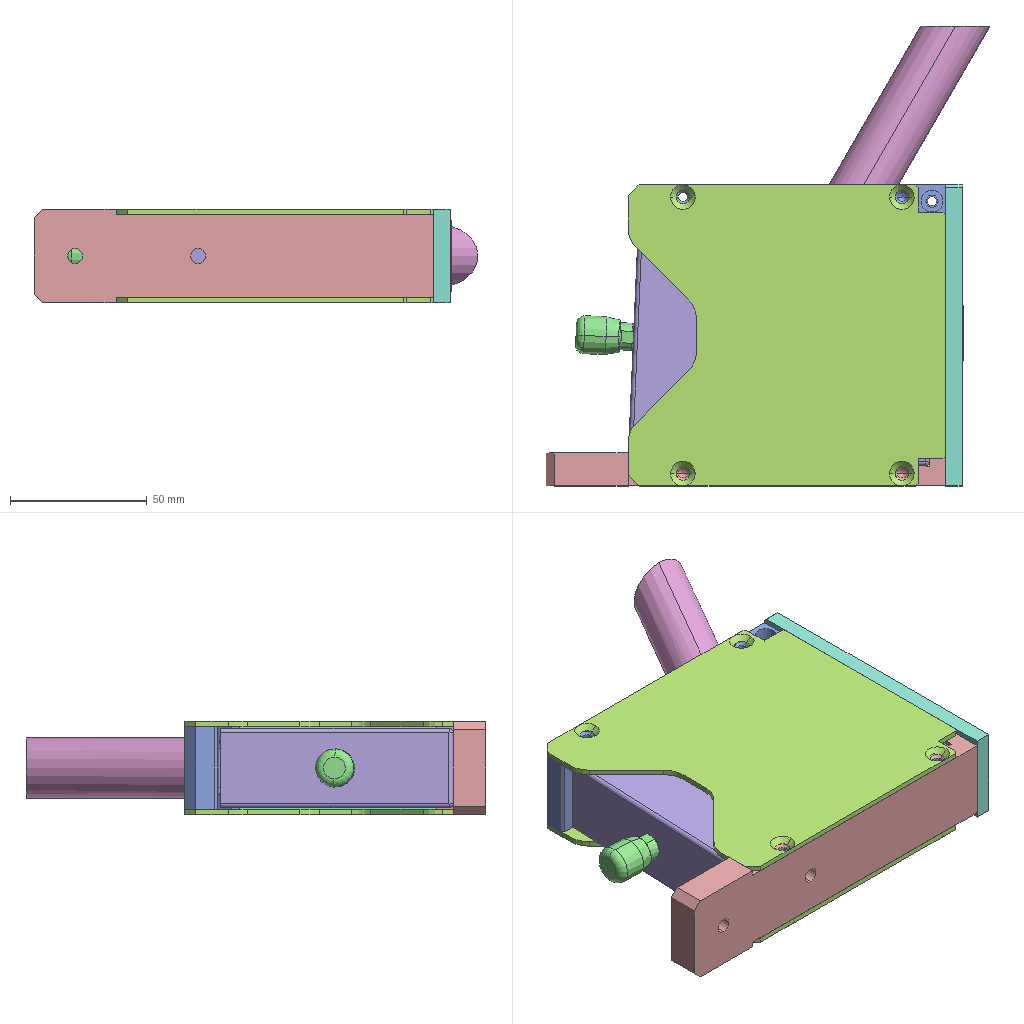Assembly | SolidWorks | 9 different items | 10 placed | box 162 x 168 x 34 mm
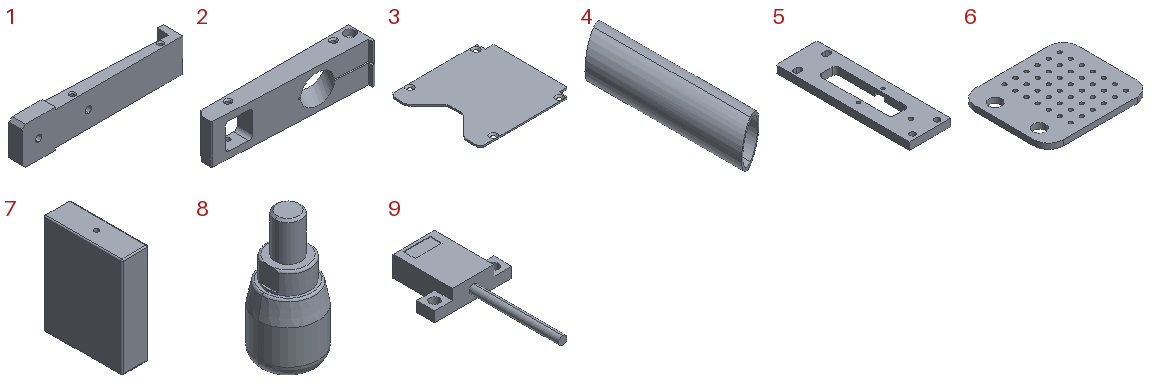Parts list (item | quantity | size | volume | features):
1 | x1 | 146 x 18 x 34 mm | 45286 mm3 | features ICE 4, HoleWzd 3, Chamfer 2, Extrusion 1, MirrorPattern 1
2 | x1 | 116 x 20 x 30 mm | 36706 mm3 | features HoleWzd 6, ICE 4, Chamfer 3, Extrusion 1, Fillet 1, MirrorPattern 1, RevCut 1
3 | x2 | 116 x 110 x 2 mm | 22518 mm3 | features Chamfer 2, ICE 2, Fillet 1, FlatPattern 1, HoleWzd 1, SMBaseFlange 1, SheetMetal 1
4 | x1 | 22 x 96 x 22 mm | 8046 mm3 | features Extrusion 1, ICE 1
5 | x1 | 34 x 110 x 6 mm | 16362 mm3 | features HoleWzd 3, ICE 3, Chamfer 1, Cut 1, Extrusion 1, Fillet 1
6 | x1 | 28 x 24 x 1.5 mm | 909.055 mm3 | features HoleWzd 2, Extrusion 1, Fillet 1, LPattern 1
7 | x1 | 29 x 85 x 110 mm | 26099 mm3 | features Extrusion 1, Fillet 1, HoleWzd 1, ICE 1, Shell 1
8 | x1 | 14 x 14 x 30 mm | 2911 mm3 | features Fillet 3, ICE 3, Chamfer 2, Extrusion 1
9 | x1 | 26 x 50.2 x 7 mm | 2334 mm3 | features ICE 4, Extrusion 1
Mates (type | each side: item.copy, entity, surface, feature):
Coincident | 1.1 face plane Cut-Extrude1 | 3.1 face plane Base-Flange1 | 2 times
Coincident | 1.1 face plane Boss-Extrude1 | 3.1 face plane Base-Flange1
Concentric | 1.1 face cylinder M4 Tapped Hole2 | 5.1 face cylinder Ø4.5 (4.5) Diameter Hole1 | 2 times
Coincident | 1.1 face plane Boss-Extrude1 | 5.1 face plane Boss-Extrude1
Width | 2.1 face plane Boss-Extrude1 | 2.1 face plane Boss-Extrude1 | 7.1 face plane Boss-Extrude1 | 7.1 face plane Boss-Extrude1
Coincident | 1.1 face plane Cut-Extrude2 | 7.1 face plane Boss-Extrude1
Coincident | 1.1 face plane Cut-Extrude3 | 7.1 face plane Boss-Extrude1
Width | 2.1 face plane Boss-Extrude1 | 2.1 face plane Boss-Extrude1 | 1.1 face plane Boss-Extrude1 | 1.1 face plane Boss-Extrude1
Coincident | 2.1 face plane Boss-Extrude1 | 5.1 face plane Boss-Extrude1 | 2 times
Concentric | 2.1 face cylinder Cut-Revolve1 | 4.1 face cylinder Boss-Extrude1
DistanceDim | 2.1 face plane Boss-Extrude1 | 4.1 face plane Cut-Extrude1
Coincident | 2.1 face plane Cut-Extrude5 | 6.1 face plane Boss-Extrude1 | 3 times
Concentric | 7.1 face cylinder M6 Tapped Hole1 | 8.1 face cylinder Boss-Extrude3
Coincident | 7.1 face plane Boss-Extrude1 | 8.1 face plane Boss-Extrude2
Coincident | 1.1 face plane Cut-Extrude1 | 3.2 face plane Base-Flange1 | 2 times
Coincident | 1.1 face plane Boss-Extrude1 | 3.2 face plane Base-Flange1
Concentric | 5.1 face cylinder M3 Tapped Hole1 | 9.1 face cylinder Cut-Extrude2 | 2 times
Coincident | 5.1 face plane Cut-Extrude3 | 9.1 face plane Cut-Extrude1